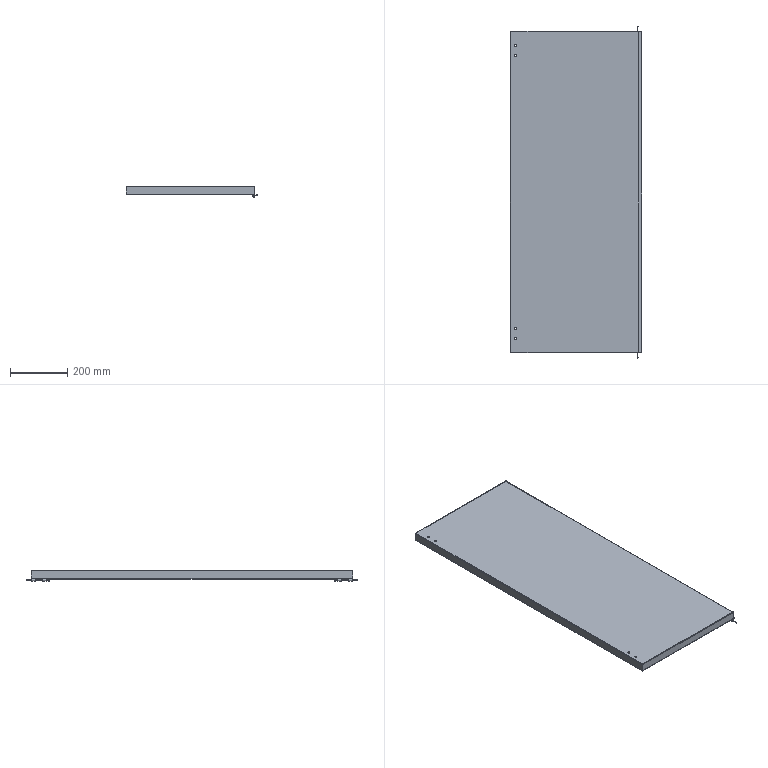Part | 5 solids | 145 faces | box 456.8 x 1156 x 41 mm | volume 748576 mm3 | plane 76 | cylinder 51 | spline 14 | torus 4 | commonest cylinder face diameters 7 x11 1.473 x8 3 x8 3.6 x8 3.873 x8 7.6 x8